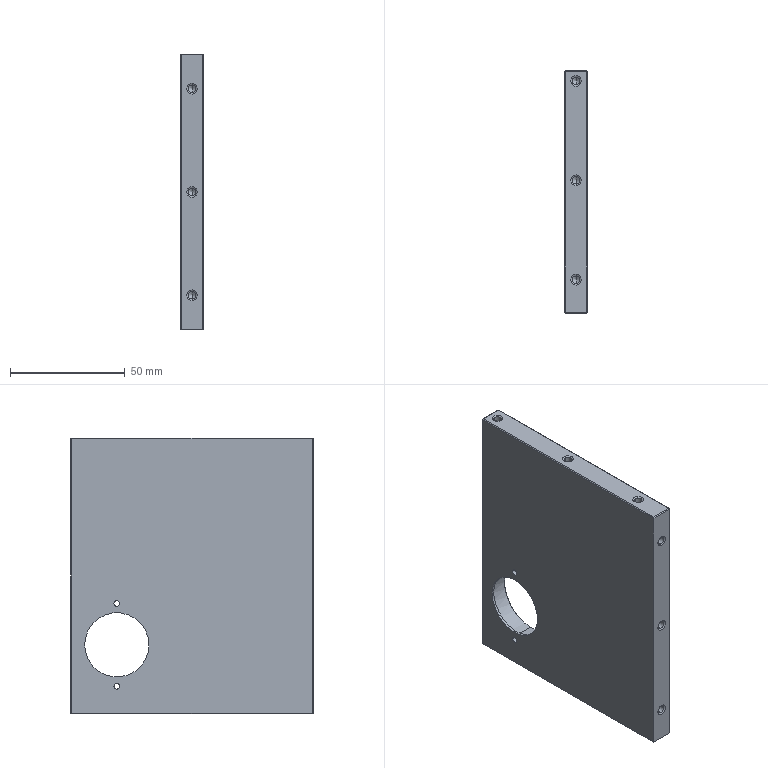Part | NX | 1 solid | 105 faces | box 10 x 105.5 x 120 mm | volume 117622 mm3 | cylinder 44 | cone 42 | plane 19 | commonest cylinder face diameters 3.3 x36 2.5 x4 28 x2 32 x2